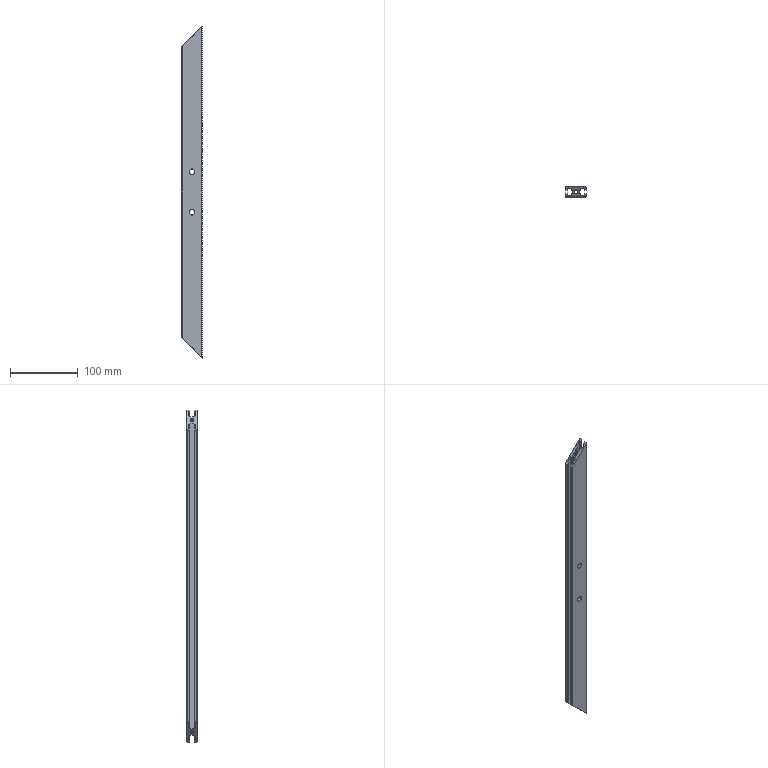Part | NX | features BREP 1 | 1 solid | 95 faces | box 30 x 15 x 491.9 mm | volume 110088 mm3 | plane 54 | cylinder 41 | commonest cylinder face diameters 1 x18 5 x15 2 x4 8.5 x4